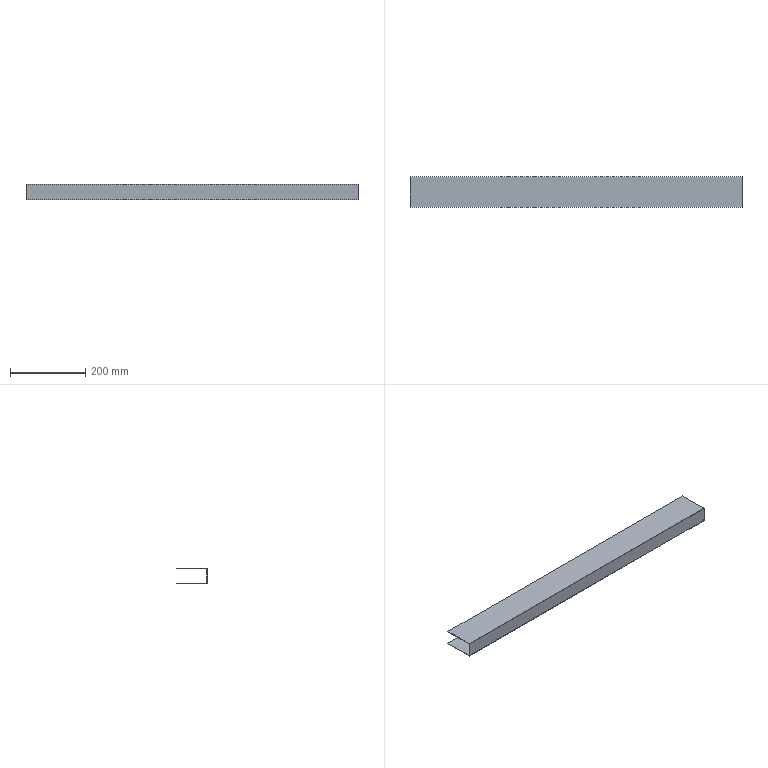Part | SolidWorks | features BaseBody 1 | 1 solid | 10 faces | box 880 x 80 x 40 mm | volume 174240 mm3 | plane 10
STEP:
#1=CARTESIAN_POINT('',(0.,1.,19.));
#2=VERTEX_POINT('',#1);
#3=CARTESIAN_POINT('',(0.,80.,19.));
#4=VERTEX_POINT('',#3);
#5=CARTESIAN_POINT('',(0.,0.,19.));
#6=DIRECTION('',(0.,1.,0.));
#7=VECTOR('',#6,1000.);
#8=LINE('',#5,#7);
#9=EDGE_CURVE('',#2,#4,#8,.T.);
#10=ORIENTED_EDGE('',*,*,#9,.F.);
#11=CARTESIAN_POINT('',(0.,1.,-19.));
#12=VERTEX_POINT('',#11);
#13=CARTESIAN_POINT('',(0.,1.,20.));
#14=DIRECTION('',(0.,0.,1.));
#15=VECTOR('',#14,1000.);
#16=LINE('',#13,#15);
#17=EDGE_CURVE('',#12,#2,#16,.T.);
#18=ORIENTED_EDGE('',*,*,#17,.F.);
#19=CARTESIAN_POINT('',(0.,80.,-19.));
#20=VERTEX_POINT('',#19);
#21=CARTESIAN_POINT('',(0.,0.,-19.));
#22=DIRECTION('',(0.,-1.,0.));
#23=VECTOR('',#22,1000.);
#24=LINE('',#21,#23);
#25=EDGE_CURVE('',#20,#12,#24,.T.);
#26=ORIENTED_EDGE('',*,*,#25,.F.);
#27=CARTESIAN_POINT('',(0.,80.,-20.));
#28=VERTEX_POINT('',#27);
#29=CARTESIAN_POINT('',(0.,80.,-19.));
#30=DIRECTION('',(0.,0.,-1.));
#31=VECTOR('',#30,1000.);
#32=LINE('',#29,#31);
#33=EDGE_CURVE('',#20,#28,#32,.T.);
#34=ORIENTED_EDGE('',*,*,#33,.T.);
#35=CARTESIAN_POINT('',(0.,0.,-20.));
#36=VERTEX_POINT('',#35);
#37=CARTESIAN_POINT('',(0.,0.,-20.));
#38=DIRECTION('',(0.,-1.,0.));
#39=VECTOR('',#38,1000.);
#40=LINE('',#37,#39);
#41=EDGE_CURVE('',#28,#36,#40,.T.);
#42=ORIENTED_EDGE('',*,*,#41,.T.);
#43=CARTESIAN_POINT('',(0.,0.,20.));
#44=VERTEX_POINT('',#43);
#45=CARTESIAN_POINT('',(0.,0.,20.));
#46=DIRECTION('',(0.,0.,1.));
#47=VECTOR('',#46,1000.);
#48=LINE('',#45,#47);
#49=EDGE_CURVE('',#36,#44,#48,.T.);
#50=ORIENTED_EDGE('',*,*,#49,.T.);
#51=CARTESIAN_POINT('',(0.,80.,20.));
#52=VERTEX_POINT('',#51);
#53=CARTESIAN_POINT('',(0.,0.,20.));
#54=DIRECTION('',(0.,1.,0.));
#55=VECTOR('',#54,1000.);
#56=LINE('',#53,#55);
#57=EDGE_CURVE('',#44,#52,#56,.T.);
#58=ORIENTED_EDGE('',*,*,#57,.T.);
#59=CARTESIAN_POINT('',(0.,80.,20.));
#60=DIRECTION('',(0.,0.,-1.));
#61=VECTOR('',#60,1000.);
#62=LINE('',#59,#61);
#63=EDGE_CURVE('',#52,#4,#62,.T.);
#64=ORIENTED_EDGE('',*,*,#63,.T.);
#65=EDGE_LOOP('',(#10,#18,#26,#34,#42,#50,#58,#64));
#66=FACE_OUTER_BOUND('',#65,.T.);
#67=CARTESIAN_POINT('',(0.,0.,0.));
#68=DIRECTION('',(-1.,0.,0.));
#69=DIRECTION('',(0.,0.,1.));
#70=AXIS2_PLACEMENT_3D('',#67,#68,#69);
#71=PLANE('',#70);
#72=ADVANCED_FACE('',(#66),#71,.T.);
#73=CARTESIAN_POINT('',(880.,1.,19.));
#74=VERTEX_POINT('',#73);
#75=CARTESIAN_POINT('',(880.,80.,19.));
#76=VERTEX_POINT('',#75);
#77=CARTESIAN_POINT('',(880.,0.,19.));
#78=DIRECTION('',(0.,1.,0.));
#79=VECTOR('',#78,1000.);
#80=LINE('',#77,#79);
#81=EDGE_CURVE('',#74,#76,#80,.T.);
#82=ORIENTED_EDGE('',*,*,#81,.T.);
#83=CARTESIAN_POINT('',(880.,80.,20.));
#84=VERTEX_POINT('',#83);
#85=CARTESIAN_POINT('',(880.,80.,20.));
#86=DIRECTION('',(0.,0.,-1.));
#87=VECTOR('',#86,1000.);
#88=LINE('',#85,#87);
#89=EDGE_CURVE('',#84,#76,#88,.T.);
#90=ORIENTED_EDGE('',*,*,#89,.F.);
#91=CARTESIAN_POINT('',(880.,0.,20.));
#92=VERTEX_POINT('',#91);
#93=CARTESIAN_POINT('',(880.,0.,20.));
#94=DIRECTION('',(0.,1.,0.));
#95=VECTOR('',#94,1000.);
#96=LINE('',#93,#95);
#97=EDGE_CURVE('',#92,#84,#96,.T.);
#98=ORIENTED_EDGE('',*,*,#97,.F.);
#99=CARTESIAN_POINT('',(880.,0.,-20.));
#100=VERTEX_POINT('',#99);
#101=CARTESIAN_POINT('',(880.,0.,20.));
#102=DIRECTION('',(0.,0.,1.));
#103=VECTOR('',#102,1000.);
#104=LINE('',#101,#103);
#105=EDGE_CURVE('',#100,#92,#104,.T.);
#106=ORIENTED_EDGE('',*,*,#105,.F.);
#107=CARTESIAN_POINT('',(880.,80.,-20.));
#108=VERTEX_POINT('',#107);
#109=CARTESIAN_POINT('',(880.,0.,-20.));
#110=DIRECTION('',(0.,-1.,0.));
#111=VECTOR('',#110,1000.);
#112=LINE('',#109,#111);
#113=EDGE_CURVE('',#108,#100,#112,.T.);
#114=ORIENTED_EDGE('',*,*,#113,.F.);
#115=CARTESIAN_POINT('',(880.,80.,-19.));
#116=VERTEX_POINT('',#115);
#117=CARTESIAN_POINT('',(880.,80.,-19.));
#118=DIRECTION('',(0.,0.,-1.));
#119=VECTOR('',#118,1000.);
#120=LINE('',#117,#119);
#121=EDGE_CURVE('',#116,#108,#120,.T.);
#122=ORIENTED_EDGE('',*,*,#121,.F.);
#123=CARTESIAN_POINT('',(880.,1.,-19.));
#124=VERTEX_POINT('',#123);
#125=CARTESIAN_POINT('',(880.,0.,-19.));
#126=DIRECTION('',(0.,-1.,0.));
#127=VECTOR('',#126,1000.);
#128=LINE('',#125,#127);
#129=EDGE_CURVE('',#116,#124,#128,.T.);
#130=ORIENTED_EDGE('',*,*,#129,.T.);
#131=CARTESIAN_POINT('',(880.,1.,20.));
#132=DIRECTION('',(0.,0.,1.));
#133=VECTOR('',#132,1000.);
#134=LINE('',#131,#133);
#135=EDGE_CURVE('',#124,#74,#134,.T.);
#136=ORIENTED_EDGE('',*,*,#135,.T.);
#137=EDGE_LOOP('',(#82,#90,#98,#106,#114,#122,#130,#136));
#138=FACE_OUTER_BOUND('',#137,.T.);
#139=CARTESIAN_POINT('',(880.,0.,0.));
#140=DIRECTION('',(-1.,0.,0.));
#141=DIRECTION('',(0.,0.,1.));
#142=AXIS2_PLACEMENT_3D('',#139,#140,#141);
#143=PLANE('',#142);
#144=ADVANCED_FACE('',(#138),#143,.F.);
#145=ORIENTED_EDGE('',*,*,#17,.T.);
#146=CARTESIAN_POINT('',(880.,1.,19.));
#147=DIRECTION('',(-1.,0.,0.));
#148=VECTOR('',#147,1000.);
#149=LINE('',#146,#148);
#150=EDGE_CURVE('',#74,#2,#149,.T.);
#151=ORIENTED_EDGE('',*,*,#150,.F.);
#152=ORIENTED_EDGE('',*,*,#135,.F.);
#153=CARTESIAN_POINT('',(880.,1.,-19.));
#154=DIRECTION('',(-1.,0.,0.));
#155=VECTOR('',#154,1000.);
#156=LINE('',#153,#155);
#157=EDGE_CURVE('',#124,#12,#156,.T.);
#158=ORIENTED_EDGE('',*,*,#157,.T.);
#159=EDGE_LOOP('',(#145,#151,#152,#158));
#160=FACE_OUTER_BOUND('',#159,.T.);
#161=CARTESIAN_POINT('',(880.,1.,20.));
#162=DIRECTION('',(0.,-1.,0.));
#163=DIRECTION('',(0.,0.,-1.));
#164=AXIS2_PLACEMENT_3D('',#161,#162,#163);
#165=PLANE('',#164);
#166=ADVANCED_FACE('',(#160),#165,.F.);
#167=ORIENTED_EDGE('',*,*,#25,.T.);
#168=ORIENTED_EDGE('',*,*,#157,.F.);
#169=ORIENTED_EDGE('',*,*,#129,.F.);
#170=CARTESIAN_POINT('',(880.,80.,-19.));
#171=DIRECTION('',(-1.,0.,0.));
#172=VECTOR('',#171,1000.);
#173=LINE('',#170,#172);
#174=EDGE_CURVE('',#116,#20,#173,.T.);
#175=ORIENTED_EDGE('',*,*,#174,.T.);
#176=EDGE_LOOP('',(#167,#168,#169,#175));
#177=FACE_OUTER_BOUND('',#176,.T.);
#178=CARTESIAN_POINT('',(880.,0.,-19.));
#179=DIRECTION('',(0.,0.,-1.));
#180=DIRECTION('',(0.,-1.,0.));
#181=AXIS2_PLACEMENT_3D('',#178,#179,#180);
#182=PLANE('',#181);
#183=ADVANCED_FACE('',(#177),#182,.F.);
#184=ORIENTED_EDGE('',*,*,#33,.F.);
#185=ORIENTED_EDGE('',*,*,#174,.F.);
#186=ORIENTED_EDGE('',*,*,#121,.T.);
#187=CARTESIAN_POINT('',(880.,80.,-20.));
#188=DIRECTION('',(-1.,0.,0.));
#189=VECTOR('',#188,1000.);
#190=LINE('',#187,#189);
#191=EDGE_CURVE('',#108,#28,#190,.T.);
#192=ORIENTED_EDGE('',*,*,#191,.T.);
#193=EDGE_LOOP('',(#184,#185,#186,#192));
#194=FACE_OUTER_BOUND('',#193,.T.);
#195=CARTESIAN_POINT('',(880.,80.,-19.));
#196=DIRECTION('',(0.,1.,0.));
#197=DIRECTION('',(1.,0.,0.));
#198=AXIS2_PLACEMENT_3D('',#195,#196,#197);
#199=PLANE('',#198);
#200=ADVANCED_FACE('',(#194),#199,.T.);
#201=ORIENTED_EDGE('',*,*,#41,.F.);
#202=ORIENTED_EDGE('',*,*,#191,.F.);
#203=ORIENTED_EDGE('',*,*,#113,.T.);
#204=CARTESIAN_POINT('',(880.,0.,-20.));
#205=DIRECTION('',(-1.,0.,0.));
#206=VECTOR('',#205,1000.);
#207=LINE('',#204,#206);
#208=EDGE_CURVE('',#100,#36,#207,.T.);
#209=ORIENTED_EDGE('',*,*,#208,.T.);
#210=EDGE_LOOP('',(#201,#202,#203,#209));
#211=FACE_OUTER_BOUND('',#210,.T.);
#212=CARTESIAN_POINT('',(880.,0.,-20.));
#213=DIRECTION('',(0.,0.,-1.));
#214=DIRECTION('',(0.,-1.,0.));
#215=AXIS2_PLACEMENT_3D('',#212,#213,#214);
#216=PLANE('',#215);
#217=ADVANCED_FACE('',(#211),#216,.T.);
#218=ORIENTED_EDGE('',*,*,#49,.F.);
#219=ORIENTED_EDGE('',*,*,#208,.F.);
#220=ORIENTED_EDGE('',*,*,#105,.T.);
#221=CARTESIAN_POINT('',(880.,0.,20.));
#222=DIRECTION('',(-1.,0.,0.));
#223=VECTOR('',#222,1000.);
#224=LINE('',#221,#223);
#225=EDGE_CURVE('',#92,#44,#224,.T.);
#226=ORIENTED_EDGE('',*,*,#225,.T.);
#227=EDGE_LOOP('',(#218,#219,#220,#226));
#228=FACE_OUTER_BOUND('',#227,.T.);
#229=CARTESIAN_POINT('',(880.,0.,20.));
#230=DIRECTION('',(0.,-1.,0.));
#231=DIRECTION('',(0.,0.,-1.));
#232=AXIS2_PLACEMENT_3D('',#229,#230,#231);
#233=PLANE('',#232);
#234=ADVANCED_FACE('',(#228),#233,.T.);
#235=ORIENTED_EDGE('',*,*,#57,.F.);
#236=ORIENTED_EDGE('',*,*,#225,.F.);
#237=ORIENTED_EDGE('',*,*,#97,.T.);
#238=CARTESIAN_POINT('',(880.,80.,20.));
#239=DIRECTION('',(-1.,0.,0.));
#240=VECTOR('',#239,1000.);
#241=LINE('',#238,#240);
#242=EDGE_CURVE('',#84,#52,#241,.T.);
#243=ORIENTED_EDGE('',*,*,#242,.T.);
#244=EDGE_LOOP('',(#235,#236,#237,#243));
#245=FACE_OUTER_BOUND('',#244,.T.);
#246=CARTESIAN_POINT('',(880.,0.,20.));
#247=DIRECTION('',(0.,0.,1.));
#248=DIRECTION('',(0.,-1.,0.));
#249=AXIS2_PLACEMENT_3D('',#246,#247,#248);
#250=PLANE('',#249);
#251=ADVANCED_FACE('',(#245),#250,.T.);
#252=ORIENTED_EDGE('',*,*,#63,.F.);
#253=ORIENTED_EDGE('',*,*,#242,.F.);
#254=ORIENTED_EDGE('',*,*,#89,.T.);
#255=CARTESIAN_POINT('',(880.,80.,19.));
#256=DIRECTION('',(-1.,0.,0.));
#257=VECTOR('',#256,1000.);
#258=LINE('',#255,#257);
#259=EDGE_CURVE('',#76,#4,#258,.T.);
#260=ORIENTED_EDGE('',*,*,#259,.T.);
#261=EDGE_LOOP('',(#252,#253,#254,#260));
#262=FACE_OUTER_BOUND('',#261,.T.);
#263=CARTESIAN_POINT('',(880.,80.,20.));
#264=DIRECTION('',(0.,1.,0.));
#265=DIRECTION('',(1.,0.,0.));
#266=AXIS2_PLACEMENT_3D('',#263,#264,#265);
#267=PLANE('',#266);
#268=ADVANCED_FACE('',(#262),#267,.T.);
#269=ORIENTED_EDGE('',*,*,#9,.T.);
#270=ORIENTED_EDGE('',*,*,#259,.F.);
#271=ORIENTED_EDGE('',*,*,#81,.F.);
#272=ORIENTED_EDGE('',*,*,#150,.T.);
#273=EDGE_LOOP('',(#269,#270,#271,#272));
#274=FACE_OUTER_BOUND('',#273,.T.);
#275=CARTESIAN_POINT('',(880.,0.,19.));
#276=DIRECTION('',(0.,0.,1.));
#277=DIRECTION('',(0.,-1.,0.));
#278=AXIS2_PLACEMENT_3D('',#275,#276,#277);
#279=PLANE('',#278);
#280=ADVANCED_FACE('',(#274),#279,.F.);
#281=CLOSED_SHELL('',(#72,#144,#166,#183,#200,#217,#234,#251,#268,#280));
#282=MANIFOLD_SOLID_BREP('',#281);
#283=CARTESIAN_POINT('',(0.,0.,0.));
#284=DIRECTION('',(0.,0.,1.));
#285=DIRECTION('',(1.,0.,0.));
#286=AXIS2_PLACEMENT_3D('',#283,#284,#285);
#287=(LENGTH_UNIT()NAMED_UNIT(*)SI_UNIT(.MILLI.,.METRE.));
#288=UNCERTAINTY_MEASURE_WITH_UNIT(LENGTH_MEASURE(0.00001),#287,'','');
#289=(NAMED_UNIT(*)PLANE_ANGLE_UNIT()SI_UNIT($,.RADIAN.));
#290=(NAMED_UNIT(*)SI_UNIT($,.STERADIAN.)SOLID_ANGLE_UNIT());
#291=(GEOMETRIC_REPRESENTATION_CONTEXT(3)GLOBAL_UNCERTAINTY_ASSIGNED_CONTEXT((#288))GLOBAL_UNIT_ASSIGNED_CONTEXT((#287,#289,#290))REPRESENTATION_CONTEXT('',''));
#292=ADVANCED_BREP_SHAPE_REPRESENTATION('',(#282,#286),#291);